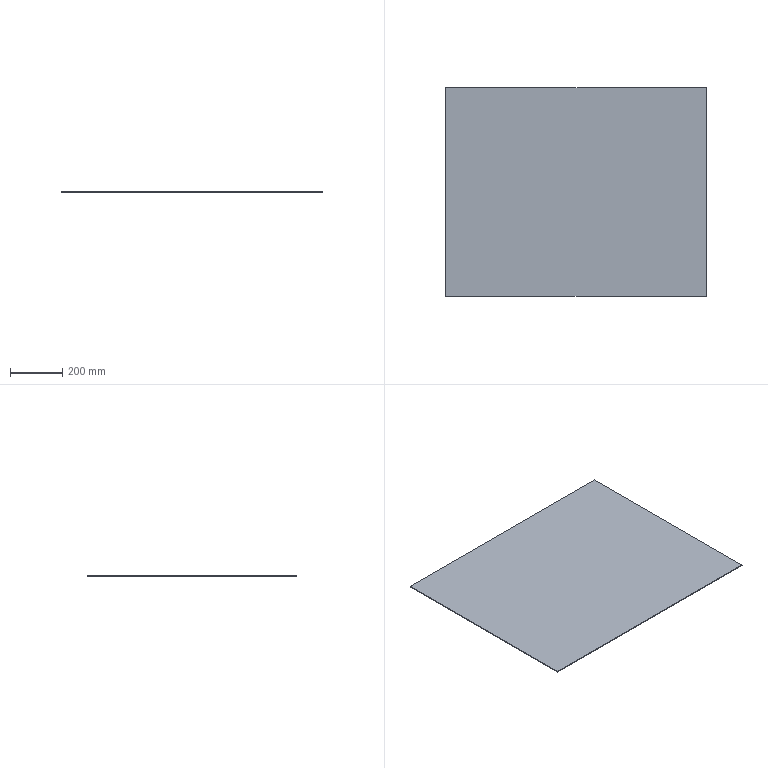Part | STEP file | Upper cover plate | 1 solid | 10 faces | box 1000 x 800 x 3 mm | volume 2399999 mm3 | plane 6 | cylinder 4 | commonest cylinder face diameters 1 x4
STEP:
#1=CARTESIAN_POINT('',(-500.,399.5,3.));
#2=VERTEX_POINT('',#1);
#3=CARTESIAN_POINT('',(-500.,-399.5,3.));
#4=VERTEX_POINT('',#3);
#5=CARTESIAN_POINT('',(-500.,400.,3.));
#6=DIRECTION('',(0.,-1.,0.));
#7=VECTOR('',#6,1000.);
#8=LINE('',#5,#7);
#9=EDGE_CURVE('',#2,#4,#8,.T.);
#10=ORIENTED_EDGE('',*,*,#9,.F.);
#11=CARTESIAN_POINT('',(-500.,399.5,0.));
#12=VERTEX_POINT('',#11);
#13=CARTESIAN_POINT('',(-500.,399.5,3.));
#14=DIRECTION('',(0.,0.,-1.));
#15=VECTOR('',#14,1000.);
#16=LINE('',#13,#15);
#17=EDGE_CURVE('',#2,#12,#16,.T.);
#18=ORIENTED_EDGE('',*,*,#17,.T.);
#19=CARTESIAN_POINT('',(-500.,-399.5,0.));
#20=VERTEX_POINT('',#19);
#21=CARTESIAN_POINT('',(-500.,400.,0.));
#22=DIRECTION('',(0.,-1.,0.));
#23=VECTOR('',#22,1000.);
#24=LINE('',#21,#23);
#25=EDGE_CURVE('',#12,#20,#24,.T.);
#26=ORIENTED_EDGE('',*,*,#25,.T.);
#27=CARTESIAN_POINT('',(-500.,-399.5,3.));
#28=DIRECTION('',(0.,0.,1.));
#29=VECTOR('',#28,1000.);
#30=LINE('',#27,#29);
#31=EDGE_CURVE('',#20,#4,#30,.T.);
#32=ORIENTED_EDGE('',*,*,#31,.T.);
#33=EDGE_LOOP('',(#10,#18,#26,#32));
#34=FACE_OUTER_BOUND('',#33,.T.);
#35=CARTESIAN_POINT('',(-500.,400.,3.));
#36=DIRECTION('',(1.,0.,0.));
#37=DIRECTION('',(0.,1.,0.));
#38=AXIS2_PLACEMENT_3D('',#35,#36,#37);
#39=PLANE('',#38);
#40=ADVANCED_FACE('',(#34),#39,.F.);
#41=CARTESIAN_POINT('',(-499.5,-400.,3.));
#42=VERTEX_POINT('',#41);
#43=CARTESIAN_POINT('',(499.5,-400.,3.));
#44=VERTEX_POINT('',#43);
#45=CARTESIAN_POINT('',(-500.,-400.,3.));
#46=DIRECTION('',(1.,0.,0.));
#47=VECTOR('',#46,1000.);
#48=LINE('',#45,#47);
#49=EDGE_CURVE('',#42,#44,#48,.T.);
#50=ORIENTED_EDGE('',*,*,#49,.F.);
#51=CARTESIAN_POINT('',(-499.5,-400.,0.));
#52=VERTEX_POINT('',#51);
#53=CARTESIAN_POINT('',(-499.5,-400.,3.));
#54=DIRECTION('',(0.,0.,-1.));
#55=VECTOR('',#54,1000.);
#56=LINE('',#53,#55);
#57=EDGE_CURVE('',#42,#52,#56,.T.);
#58=ORIENTED_EDGE('',*,*,#57,.T.);
#59=CARTESIAN_POINT('',(499.5,-400.,0.));
#60=VERTEX_POINT('',#59);
#61=CARTESIAN_POINT('',(-500.,-400.,0.));
#62=DIRECTION('',(1.,0.,0.));
#63=VECTOR('',#62,1000.);
#64=LINE('',#61,#63);
#65=EDGE_CURVE('',#52,#60,#64,.T.);
#66=ORIENTED_EDGE('',*,*,#65,.T.);
#67=CARTESIAN_POINT('',(499.5,-400.,3.));
#68=DIRECTION('',(0.,0.,1.));
#69=VECTOR('',#68,1000.);
#70=LINE('',#67,#69);
#71=EDGE_CURVE('',#60,#44,#70,.T.);
#72=ORIENTED_EDGE('',*,*,#71,.T.);
#73=EDGE_LOOP('',(#50,#58,#66,#72));
#74=FACE_OUTER_BOUND('',#73,.T.);
#75=CARTESIAN_POINT('',(-500.,-400.,3.));
#76=DIRECTION('',(0.,1.,0.));
#77=DIRECTION('',(0.,0.,1.));
#78=AXIS2_PLACEMENT_3D('',#75,#76,#77);
#79=PLANE('',#78);
#80=ADVANCED_FACE('',(#74),#79,.F.);
#81=CARTESIAN_POINT('',(500.,-399.5,0.));
#82=VERTEX_POINT('',#81);
#83=CARTESIAN_POINT('',(500.,399.5,0.));
#84=VERTEX_POINT('',#83);
#85=CARTESIAN_POINT('',(500.,400.,0.));
#86=DIRECTION('',(0.,1.,0.));
#87=VECTOR('',#86,1000.);
#88=LINE('',#85,#87);
#89=EDGE_CURVE('',#82,#84,#88,.T.);
#90=ORIENTED_EDGE('',*,*,#89,.T.);
#91=CARTESIAN_POINT('',(500.,399.5,3.));
#92=VERTEX_POINT('',#91);
#93=CARTESIAN_POINT('',(500.,399.5,3.));
#94=DIRECTION('',(0.,0.,1.));
#95=VECTOR('',#94,1000.);
#96=LINE('',#93,#95);
#97=EDGE_CURVE('',#84,#92,#96,.T.);
#98=ORIENTED_EDGE('',*,*,#97,.T.);
#99=CARTESIAN_POINT('',(500.,-399.5,3.));
#100=VERTEX_POINT('',#99);
#101=CARTESIAN_POINT('',(500.,400.,3.));
#102=DIRECTION('',(0.,1.,0.));
#103=VECTOR('',#102,1000.);
#104=LINE('',#101,#103);
#105=EDGE_CURVE('',#100,#92,#104,.T.);
#106=ORIENTED_EDGE('',*,*,#105,.F.);
#107=CARTESIAN_POINT('',(500.,-399.5,3.));
#108=DIRECTION('',(0.,0.,-1.));
#109=VECTOR('',#108,1000.);
#110=LINE('',#107,#109);
#111=EDGE_CURVE('',#100,#82,#110,.T.);
#112=ORIENTED_EDGE('',*,*,#111,.T.);
#113=EDGE_LOOP('',(#90,#98,#106,#112));
#114=FACE_OUTER_BOUND('',#113,.T.);
#115=CARTESIAN_POINT('',(500.,400.,3.));
#116=DIRECTION('',(-1.,0.,0.));
#117=DIRECTION('',(0.,-1.,0.));
#118=AXIS2_PLACEMENT_3D('',#115,#116,#117);
#119=PLANE('',#118);
#120=ADVANCED_FACE('',(#114),#119,.F.);
#121=CARTESIAN_POINT('',(499.5,400.,3.));
#122=VERTEX_POINT('',#121);
#123=CARTESIAN_POINT('',(-499.5,400.,3.));
#124=VERTEX_POINT('',#123);
#125=CARTESIAN_POINT('',(-500.,400.,3.));
#126=DIRECTION('',(-1.,0.,0.));
#127=VECTOR('',#126,1000.);
#128=LINE('',#125,#127);
#129=EDGE_CURVE('',#122,#124,#128,.T.);
#130=ORIENTED_EDGE('',*,*,#129,.F.);
#131=CARTESIAN_POINT('',(499.5,400.,0.));
#132=VERTEX_POINT('',#131);
#133=CARTESIAN_POINT('',(499.5,400.,3.));
#134=DIRECTION('',(0.,0.,-1.));
#135=VECTOR('',#134,1000.);
#136=LINE('',#133,#135);
#137=EDGE_CURVE('',#122,#132,#136,.T.);
#138=ORIENTED_EDGE('',*,*,#137,.T.);
#139=CARTESIAN_POINT('',(-499.5,400.,0.));
#140=VERTEX_POINT('',#139);
#141=CARTESIAN_POINT('',(-500.,400.,0.));
#142=DIRECTION('',(-1.,0.,0.));
#143=VECTOR('',#142,1000.);
#144=LINE('',#141,#143);
#145=EDGE_CURVE('',#132,#140,#144,.T.);
#146=ORIENTED_EDGE('',*,*,#145,.T.);
#147=CARTESIAN_POINT('',(-499.5,400.,3.));
#148=DIRECTION('',(0.,0.,1.));
#149=VECTOR('',#148,1000.);
#150=LINE('',#147,#149);
#151=EDGE_CURVE('',#140,#124,#150,.T.);
#152=ORIENTED_EDGE('',*,*,#151,.T.);
#153=EDGE_LOOP('',(#130,#138,#146,#152));
#154=FACE_OUTER_BOUND('',#153,.T.);
#155=CARTESIAN_POINT('',(-500.,400.,3.));
#156=DIRECTION('',(0.,-1.,0.));
#157=DIRECTION('',(0.,0.,-1.));
#158=AXIS2_PLACEMENT_3D('',#155,#156,#157);
#159=PLANE('',#158);
#160=ADVANCED_FACE('',(#154),#159,.F.);
#161=ORIENTED_EDGE('',*,*,#105,.T.);
#162=CARTESIAN_POINT('',(499.5,399.5,3.));
#163=DIRECTION('',(0.,0.,1.));
#164=DIRECTION('',(1.,0.,0.));
#165=AXIS2_PLACEMENT_3D('',#162,#163,#164);
#166=CIRCLE('',#165,0.5);
#167=EDGE_CURVE('',#92,#122,#166,.T.);
#168=ORIENTED_EDGE('',*,*,#167,.T.);
#169=ORIENTED_EDGE('',*,*,#129,.T.);
#170=CARTESIAN_POINT('',(-499.5,399.5,3.));
#171=DIRECTION('',(0.,0.,1.));
#172=DIRECTION('',(1.,0.,0.));
#173=AXIS2_PLACEMENT_3D('',#170,#171,#172);
#174=CIRCLE('',#173,0.5);
#175=EDGE_CURVE('',#124,#2,#174,.T.);
#176=ORIENTED_EDGE('',*,*,#175,.T.);
#177=ORIENTED_EDGE('',*,*,#9,.T.);
#178=CARTESIAN_POINT('',(-499.5,-399.5,3.));
#179=DIRECTION('',(0.,0.,1.));
#180=DIRECTION('',(1.,0.,0.));
#181=AXIS2_PLACEMENT_3D('',#178,#179,#180);
#182=CIRCLE('',#181,0.5);
#183=EDGE_CURVE('',#4,#42,#182,.T.);
#184=ORIENTED_EDGE('',*,*,#183,.T.);
#185=ORIENTED_EDGE('',*,*,#49,.T.);
#186=CARTESIAN_POINT('',(499.5,-399.5,3.));
#187=DIRECTION('',(0.,0.,1.));
#188=DIRECTION('',(1.,0.,0.));
#189=AXIS2_PLACEMENT_3D('',#186,#187,#188);
#190=CIRCLE('',#189,0.5);
#191=EDGE_CURVE('',#44,#100,#190,.T.);
#192=ORIENTED_EDGE('',*,*,#191,.T.);
#193=EDGE_LOOP('',(#161,#168,#169,#176,#177,#184,#185,#192));
#194=FACE_OUTER_BOUND('',#193,.T.);
#195=CARTESIAN_POINT('',(0.,0.,3.));
#196=DIRECTION('',(0.,0.,1.));
#197=DIRECTION('',(1.,0.,0.));
#198=AXIS2_PLACEMENT_3D('',#195,#196,#197);
#199=PLANE('',#198);
#200=ADVANCED_FACE('',(#194),#199,.T.);
#201=ORIENTED_EDGE('',*,*,#145,.F.);
#202=CARTESIAN_POINT('',(499.5,399.5,0.));
#203=DIRECTION('',(0.,0.,-1.));
#204=DIRECTION('',(1.,0.,0.));
#205=AXIS2_PLACEMENT_3D('',#202,#203,#204);
#206=CIRCLE('',#205,0.5);
#207=EDGE_CURVE('',#132,#84,#206,.T.);
#208=ORIENTED_EDGE('',*,*,#207,.T.);
#209=ORIENTED_EDGE('',*,*,#89,.F.);
#210=CARTESIAN_POINT('',(499.5,-399.5,0.));
#211=DIRECTION('',(0.,0.,-1.));
#212=DIRECTION('',(1.,0.,0.));
#213=AXIS2_PLACEMENT_3D('',#210,#211,#212);
#214=CIRCLE('',#213,0.5);
#215=EDGE_CURVE('',#82,#60,#214,.T.);
#216=ORIENTED_EDGE('',*,*,#215,.T.);
#217=ORIENTED_EDGE('',*,*,#65,.F.);
#218=CARTESIAN_POINT('',(-499.5,-399.5,0.));
#219=DIRECTION('',(0.,0.,-1.));
#220=DIRECTION('',(1.,0.,0.));
#221=AXIS2_PLACEMENT_3D('',#218,#219,#220);
#222=CIRCLE('',#221,0.5);
#223=EDGE_CURVE('',#52,#20,#222,.T.);
#224=ORIENTED_EDGE('',*,*,#223,.T.);
#225=ORIENTED_EDGE('',*,*,#25,.F.);
#226=CARTESIAN_POINT('',(-499.5,399.5,0.));
#227=DIRECTION('',(0.,0.,-1.));
#228=DIRECTION('',(1.,0.,0.));
#229=AXIS2_PLACEMENT_3D('',#226,#227,#228);
#230=CIRCLE('',#229,0.5);
#231=EDGE_CURVE('',#12,#140,#230,.T.);
#232=ORIENTED_EDGE('',*,*,#231,.T.);
#233=EDGE_LOOP('',(#201,#208,#209,#216,#217,#224,#225,#232));
#234=FACE_OUTER_BOUND('',#233,.T.);
#235=CARTESIAN_POINT('',(0.,0.,0.));
#236=DIRECTION('',(0.,0.,1.));
#237=DIRECTION('',(1.,0.,0.));
#238=AXIS2_PLACEMENT_3D('',#235,#236,#237);
#239=PLANE('',#238);
#240=ADVANCED_FACE('',(#234),#239,.F.);
#241=ORIENTED_EDGE('',*,*,#167,.F.);
#242=ORIENTED_EDGE('',*,*,#97,.F.);
#243=ORIENTED_EDGE('',*,*,#207,.F.);
#244=ORIENTED_EDGE('',*,*,#137,.F.);
#245=EDGE_LOOP('',(#241,#242,#243,#244));
#246=FACE_OUTER_BOUND('',#245,.T.);
#247=CARTESIAN_POINT('',(499.5,399.5,3.));
#248=DIRECTION('',(0.,0.,-1.));
#249=DIRECTION('',(-1.,0.,0.));
#250=AXIS2_PLACEMENT_3D('',#247,#248,#249);
#251=CYLINDRICAL_SURFACE('',#250,0.5);
#252=ADVANCED_FACE('',(#246),#251,.T.);
#253=ORIENTED_EDGE('',*,*,#175,.F.);
#254=ORIENTED_EDGE('',*,*,#151,.F.);
#255=ORIENTED_EDGE('',*,*,#231,.F.);
#256=ORIENTED_EDGE('',*,*,#17,.F.);
#257=EDGE_LOOP('',(#253,#254,#255,#256));
#258=FACE_OUTER_BOUND('',#257,.T.);
#259=CARTESIAN_POINT('',(-499.5,399.5,3.));
#260=DIRECTION('',(0.,0.,-1.));
#261=DIRECTION('',(-1.,0.,0.));
#262=AXIS2_PLACEMENT_3D('',#259,#260,#261);
#263=CYLINDRICAL_SURFACE('',#262,0.5);
#264=ADVANCED_FACE('',(#258),#263,.T.);
#265=ORIENTED_EDGE('',*,*,#183,.F.);
#266=ORIENTED_EDGE('',*,*,#31,.F.);
#267=ORIENTED_EDGE('',*,*,#223,.F.);
#268=ORIENTED_EDGE('',*,*,#57,.F.);
#269=EDGE_LOOP('',(#265,#266,#267,#268));
#270=FACE_OUTER_BOUND('',#269,.T.);
#271=CARTESIAN_POINT('',(-499.5,-399.5,3.));
#272=DIRECTION('',(0.,0.,-1.));
#273=DIRECTION('',(-1.,0.,0.));
#274=AXIS2_PLACEMENT_3D('',#271,#272,#273);
#275=CYLINDRICAL_SURFACE('',#274,0.5);
#276=ADVANCED_FACE('',(#270),#275,.T.);
#277=ORIENTED_EDGE('',*,*,#191,.F.);
#278=ORIENTED_EDGE('',*,*,#71,.F.);
#279=ORIENTED_EDGE('',*,*,#215,.F.);
#280=ORIENTED_EDGE('',*,*,#111,.F.);
#281=EDGE_LOOP('',(#277,#278,#279,#280));
#282=FACE_OUTER_BOUND('',#281,.T.);
#283=CARTESIAN_POINT('',(499.5,-399.5,3.));
#284=DIRECTION('',(0.,0.,-1.));
#285=DIRECTION('',(-1.,0.,0.));
#286=AXIS2_PLACEMENT_3D('',#283,#284,#285);
#287=CYLINDRICAL_SURFACE('',#286,0.5);
#288=ADVANCED_FACE('',(#282),#287,.T.);
#289=CLOSED_SHELL('',(#40,#80,#120,#160,#200,#240,#252,#264,#276,#288));
#290=MANIFOLD_SOLID_BREP('',#289);
#291=CARTESIAN_POINT('',(0.,0.,0.));
#292=DIRECTION('',(0.,0.,1.));
#293=DIRECTION('',(1.,0.,0.));
#294=AXIS2_PLACEMENT_3D('',#291,#292,#293);
#295=(LENGTH_UNIT()NAMED_UNIT(*)SI_UNIT(.MILLI.,.METRE.));
#296=UNCERTAINTY_MEASURE_WITH_UNIT(LENGTH_MEASURE(0.00001),#295,'','');
#297=(NAMED_UNIT(*)PLANE_ANGLE_UNIT()SI_UNIT($,.RADIAN.));
#298=(NAMED_UNIT(*)SI_UNIT($,.STERADIAN.)SOLID_ANGLE_UNIT());
#299=(GEOMETRIC_REPRESENTATION_CONTEXT(3)GLOBAL_UNCERTAINTY_ASSIGNED_CONTEXT((#296))GLOBAL_UNIT_ASSIGNED_CONTEXT((#295,#297,#298))REPRESENTATION_CONTEXT('',''));
#300=ADVANCED_BREP_SHAPE_REPRESENTATION('',(#290,#294),#299);